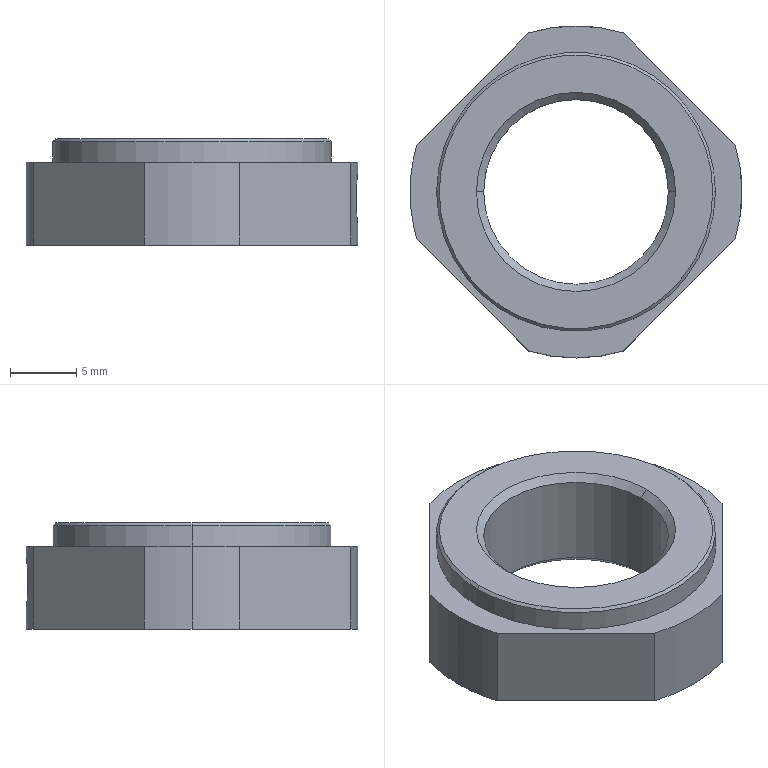Part | NX | features BREP 1 | 1 solid | 34 faces | box 25 x 25 x 8 mm | volume 2054 mm3 | cylinder 13 | cone 12 | plane 9 | commonest cylinder face diameters 25 x5 3.242 x4 13.917 x2 21 x2
STEP:
#1=CARTESIAN_POINT('',(0.,12.121,1.879));
#2=VERTEX_POINT('',#1);
#3=CARTESIAN_POINT('',(0.,7.228,1.879));
#4=VERTEX_POINT('',#3);
#5=CARTESIAN_POINT('',(0.,12.121,1.879));
#6=DIRECTION('',(0.,-1.,0.));
#7=VECTOR('',#6,1000.);
#8=LINE('',#5,#7);
#9=EDGE_CURVE('',#2,#4,#8,.T.);
#10=ORIENTED_EDGE('',*,*,#9,.F.);
#11=CARTESIAN_POINT('',(0.,12.121,5.121));
#12=VERTEX_POINT('',#11);
#13=CARTESIAN_POINT('',(0.,12.121,3.5));
#14=DIRECTION('',(0.,-1.,0.));
#15=DIRECTION('',(0.,0.,1.));
#16=AXIS2_PLACEMENT_3D('',#13,#14,#15);
#17=CIRCLE('',#16,1.621);
#18=EDGE_CURVE('',#12,#2,#17,.T.);
#19=ORIENTED_EDGE('',*,*,#18,.F.);
#20=CARTESIAN_POINT('',(0.,7.228,5.121));
#21=VERTEX_POINT('',#20);
#22=CARTESIAN_POINT('',(0.,12.121,5.121));
#23=DIRECTION('',(0.,-1.,0.));
#24=VECTOR('',#23,1000.);
#25=LINE('',#22,#24);
#26=EDGE_CURVE('',#12,#21,#25,.T.);
#27=ORIENTED_EDGE('',*,*,#26,.T.);
#28=CARTESIAN_POINT('',(0.,7.228,3.5));
#29=DIRECTION('',(0.,1.,0.));
#30=DIRECTION('',(0.,0.,-1.));
#31=AXIS2_PLACEMENT_3D('',#28,#29,#30);
#32=CIRCLE('',#31,1.621);
#33=EDGE_CURVE('',#4,#21,#32,.T.);
#34=ORIENTED_EDGE('',*,*,#33,.F.);
#35=EDGE_LOOP('',(#10,#19,#27,#34));
#36=FACE_BOUND('',#35,.T.);
#37=CARTESIAN_POINT('',(0.,12.5,3.5));
#38=DIRECTION('',(0.,-1.,0.));
#39=DIRECTION('',(0.,0.,1.));
#40=AXIS2_PLACEMENT_3D('',#37,#38,#39);
#41=CYLINDRICAL_SURFACE('',#40,1.621);
#42=ADVANCED_FACE('',(#36),#41,.F.);
#43=ORIENTED_EDGE('',*,*,#33,.T.);
#44=CARTESIAN_POINT('',(0.,7.228,3.5));
#45=DIRECTION('',(0.,1.,0.));
#46=DIRECTION('',(0.,0.,1.));
#47=AXIS2_PLACEMENT_3D('',#44,#45,#46);
#48=CIRCLE('',#47,1.621);
#49=EDGE_CURVE('',#21,#4,#48,.T.);
#50=ORIENTED_EDGE('',*,*,#49,.T.);
#51=EDGE_LOOP('',(#43,#50));
#52=FACE_BOUND('',#51,.T.);
#53=CARTESIAN_POINT('',(0.,7.228,3.5));
#54=DIRECTION('',(0.,1.,0.));
#55=DIRECTION('',(1.,0.,0.));
#56=AXIS2_PLACEMENT_3D('',#53,#54,#55);
#57=PLANE('',#56);
#58=ADVANCED_FACE('',(#52),#57,.T.);
#59=ORIENTED_EDGE('',*,*,#26,.F.);
#60=CARTESIAN_POINT('',(0.,12.121,3.5));
#61=DIRECTION('',(0.,-1.,0.));
#62=DIRECTION('',(0.,0.,-1.));
#63=AXIS2_PLACEMENT_3D('',#60,#61,#62);
#64=CIRCLE('',#63,1.621);
#65=EDGE_CURVE('',#2,#12,#64,.T.);
#66=ORIENTED_EDGE('',*,*,#65,.F.);
#67=ORIENTED_EDGE('',*,*,#9,.T.);
#68=ORIENTED_EDGE('',*,*,#49,.F.);
#69=EDGE_LOOP('',(#59,#66,#67,#68));
#70=FACE_BOUND('',#69,.T.);
#71=CARTESIAN_POINT('',(0.,12.5,3.5));
#72=DIRECTION('',(0.,-1.,0.));
#73=DIRECTION('',(0.,0.,1.));
#74=AXIS2_PLACEMENT_3D('',#71,#72,#73);
#75=CYLINDRICAL_SURFACE('',#74,1.621);
#76=ADVANCED_FACE('',(#70),#75,.F.);
#77=CARTESIAN_POINT('',(-0.0004841,12.5,1.5));
#78=VERTEX_POINT('',#77);
#79=CARTESIAN_POINT('',(0.,12.121,1.879));
#80=CARTESIAN_POINT('',(-0.000003277,12.247,1.753));
#81=CARTESIAN_POINT('',(-0.000007319,12.374,1.626));
#82=CARTESIAN_POINT('',(-0.00001213,12.5,1.5));
#83=B_SPLINE_CURVE_WITH_KNOTS('',3,(#79,#80,#81,#82),.UNSPECIFIED.,.F.,.F.,(4,4),(0.,1.),.UNSPECIFIED.);
#84=EDGE_CURVE('',#78,#2,#83,.F.);
#85=ORIENTED_EDGE('',*,*,#84,.T.);
#86=ORIENTED_EDGE('',*,*,#65,.T.);
#87=CARTESIAN_POINT('',(-0.000000003,12.5,5.5));
#88=VERTEX_POINT('',#87);
#89=CARTESIAN_POINT('',(0.,12.121,5.121));
#90=DIRECTION('',(-0.000000005,0.7071,0.7071));
#91=VECTOR('',#90,1000.);
#92=LINE('',#89,#91);
#93=EDGE_CURVE('',#88,#12,#92,.F.);
#94=ORIENTED_EDGE('',*,*,#93,.F.);
#95=CARTESIAN_POINT('',(1.356,12.426,4.868));
#96=VERTEX_POINT('',#95);
#97=CARTESIAN_POINT('',(1.356,12.426,4.868));
#98=CARTESIAN_POINT('',(0.9975,12.465,5.279));
#99=CARTESIAN_POINT('',(0.5025,12.5,5.5));
#100=CARTESIAN_POINT('',(-0.000000003,12.5,5.5));
#101=B_SPLINE_CURVE_WITH_KNOTS('',3,(#97,#98,#99,#100),.UNSPECIFIED.,.F.,.F.,(4,4),(0.,1.),.UNSPECIFIED.);
#102=EDGE_CURVE('',#96,#88,#101,.T.);
#103=ORIENTED_EDGE('',*,*,#102,.F.);
#104=CARTESIAN_POINT('',(-0.00001213,12.5,1.5));
#105=CARTESIAN_POINT('',(0.6876,12.5,1.5));
#106=CARTESIAN_POINT('',(2.094,12.337,2.407));
#107=CARTESIAN_POINT('',(1.861,12.371,4.289));
#108=CARTESIAN_POINT('',(1.356,12.426,4.868));
#109=B_SPLINE_CURVE_WITH_KNOTS('',3,(#104,#105,#106,#107,#108),.UNSPECIFIED.,.F.,.F.,(4,1,4),(0.,0.5,1.),.UNSPECIFIED.);
#110=EDGE_CURVE('',#78,#96,#109,.T.);
#111=ORIENTED_EDGE('',*,*,#110,.F.);
#112=EDGE_LOOP('',(#85,#86,#94,#103,#111));
#113=FACE_BOUND('',#112,.T.);
#114=CARTESIAN_POINT('',(0.,12.311,3.5));
#115=DIRECTION('',(0.,1.,0.));
#116=DIRECTION('',(0.,0.,1.));
#117=AXIS2_PLACEMENT_3D('',#114,#115,#116);
#118=CONICAL_SURFACE('',#117,1.811,0.7854);
#119=ADVANCED_FACE('',(#113),#118,.F.);
#120=CARTESIAN_POINT('',(-3.58,11.976,0.));
#121=VERTEX_POINT('',#120);
#122=CARTESIAN_POINT('',(-3.58,11.976,6.25));
#123=VERTEX_POINT('',#122);
#124=CARTESIAN_POINT('',(-3.58,11.976,0.));
#125=DIRECTION('',(0.,0.,1.));
#126=VECTOR('',#125,1000.);
#127=LINE('',#124,#126);
#128=EDGE_CURVE('',#121,#123,#127,.T.);
#129=ORIENTED_EDGE('',*,*,#128,.T.);
#130=CARTESIAN_POINT('',(3.58,11.976,6.25));
#131=VERTEX_POINT('',#130);
#132=CARTESIAN_POINT('',(0.,0.,6.25));
#133=DIRECTION('',(0.,0.,1.));
#134=DIRECTION('',(0.2864,0.9581,0.));
#135=AXIS2_PLACEMENT_3D('',#132,#133,#134);
#136=CIRCLE('',#135,12.5);
#137=EDGE_CURVE('',#131,#123,#136,.T.);
#138=ORIENTED_EDGE('',*,*,#137,.F.);
#139=CARTESIAN_POINT('',(3.58,11.976,0.));
#140=VERTEX_POINT('',#139);
#141=CARTESIAN_POINT('',(3.58,11.976,6.25));
#142=DIRECTION('',(0.,0.,-1.));
#143=VECTOR('',#142,1000.);
#144=LINE('',#141,#143);
#145=EDGE_CURVE('',#131,#140,#144,.T.);
#146=ORIENTED_EDGE('',*,*,#145,.T.);
#147=CARTESIAN_POINT('',(0.,0.,0.));
#148=DIRECTION('',(0.,0.,-1.));
#149=DIRECTION('',(-0.2864,0.9581,0.));
#150=AXIS2_PLACEMENT_3D('',#147,#148,#149);
#151=CIRCLE('',#150,12.5);
#152=EDGE_CURVE('',#121,#140,#151,.T.);
#153=ORIENTED_EDGE('',*,*,#152,.F.);
#154=EDGE_LOOP('',(#129,#138,#146,#153));
#155=FACE_BOUND('',#154,.T.);
#156=ORIENTED_EDGE('',*,*,#102,.T.);
#157=CARTESIAN_POINT('',(-1.357,12.426,2.134));
#158=VERTEX_POINT('',#157);
#159=CARTESIAN_POINT('',(-0.000000003,12.5,5.5));
#160=CARTESIAN_POINT('',(-0.6839,12.5,5.5));
#161=CARTESIAN_POINT('',(-2.094,12.337,4.589));
#162=CARTESIAN_POINT('',(-1.865,12.371,2.716));
#163=CARTESIAN_POINT('',(-1.357,12.426,2.134));
#164=B_SPLINE_CURVE_WITH_KNOTS('',3,(#159,#160,#161,#162,#163),.UNSPECIFIED.,.F.,.F.,(4,1,4),(0.,0.5,1.),.UNSPECIFIED.);
#165=EDGE_CURVE('',#88,#158,#164,.T.);
#166=ORIENTED_EDGE('',*,*,#165,.T.);
#167=CARTESIAN_POINT('',(-1.357,12.426,2.134));
#168=CARTESIAN_POINT('',(-1.003,12.465,1.727));
#169=CARTESIAN_POINT('',(-0.5062,12.5,1.5));
#170=CARTESIAN_POINT('',(-0.0004841,12.5,1.5));
#171=B_SPLINE_CURVE_WITH_KNOTS('',3,(#167,#168,#169,#170),.UNSPECIFIED.,.F.,.F.,(4,4),(0.,0.9997),.UNSPECIFIED.);
#172=EDGE_CURVE('',#158,#78,#171,.T.);
#173=ORIENTED_EDGE('',*,*,#172,.T.);
#174=ORIENTED_EDGE('',*,*,#110,.T.);
#175=EDGE_LOOP('',(#156,#166,#173,#174));
#176=FACE_BOUND('',#175,.T.);
#177=CARTESIAN_POINT('',(0.,0.,6.25));
#178=DIRECTION('',(0.,0.,1.));
#179=DIRECTION('',(-1.,0.,0.));
#180=AXIS2_PLACEMENT_3D('',#177,#178,#179);
#181=CYLINDRICAL_SURFACE('',#180,12.5);
#182=ADVANCED_FACE('',(#155,#176),#181,.T.);
#183=ORIENTED_EDGE('',*,*,#152,.T.);
#184=CARTESIAN_POINT('',(11.976,3.58,0.));
#185=VERTEX_POINT('',#184);
#186=CARTESIAN_POINT('',(3.58,11.976,0.));
#187=DIRECTION('',(0.7071,-0.7071,0.));
#188=VECTOR('',#187,1000.);
#189=LINE('',#186,#188);
#190=EDGE_CURVE('',#140,#185,#189,.T.);
#191=ORIENTED_EDGE('',*,*,#190,.T.);
#192=CARTESIAN_POINT('',(11.976,-3.58,0.));
#193=VERTEX_POINT('',#192);
#194=CARTESIAN_POINT('',(0.,0.,0.));
#195=DIRECTION('',(0.,0.,-1.));
#196=DIRECTION('',(0.9581,0.2864,0.));
#197=AXIS2_PLACEMENT_3D('',#194,#195,#196);
#198=CIRCLE('',#197,12.5);
#199=EDGE_CURVE('',#185,#193,#198,.T.);
#200=ORIENTED_EDGE('',*,*,#199,.T.);
#201=CARTESIAN_POINT('',(3.58,-11.976,0.));
#202=VERTEX_POINT('',#201);
#203=CARTESIAN_POINT('',(11.976,-3.58,0.));
#204=DIRECTION('',(-0.7071,-0.7071,0.));
#205=VECTOR('',#204,1000.);
#206=LINE('',#203,#205);
#207=EDGE_CURVE('',#193,#202,#206,.T.);
#208=ORIENTED_EDGE('',*,*,#207,.T.);
#209=CARTESIAN_POINT('',(-3.58,-11.976,0.));
#210=VERTEX_POINT('',#209);
#211=CARTESIAN_POINT('',(0.,0.,0.));
#212=DIRECTION('',(0.,0.,-1.));
#213=DIRECTION('',(0.2864,-0.9581,0.));
#214=AXIS2_PLACEMENT_3D('',#211,#212,#213);
#215=CIRCLE('',#214,12.5);
#216=EDGE_CURVE('',#202,#210,#215,.T.);
#217=ORIENTED_EDGE('',*,*,#216,.T.);
#218=CARTESIAN_POINT('',(-11.976,-3.58,0.));
#219=VERTEX_POINT('',#218);
#220=CARTESIAN_POINT('',(-3.58,-11.976,0.));
#221=DIRECTION('',(-0.7071,0.7071,0.));
#222=VECTOR('',#221,1000.);
#223=LINE('',#220,#222);
#224=EDGE_CURVE('',#210,#219,#223,.T.);
#225=ORIENTED_EDGE('',*,*,#224,.T.);
#226=CARTESIAN_POINT('',(-12.5,0.,0.));
#227=VERTEX_POINT('',#226);
#228=CARTESIAN_POINT('',(0.,0.,0.));
#229=DIRECTION('',(0.,0.,-1.));
#230=DIRECTION('',(-0.9581,-0.2864,0.));
#231=AXIS2_PLACEMENT_3D('',#228,#229,#230);
#232=CIRCLE('',#231,12.5);
#233=EDGE_CURVE('',#219,#227,#232,.T.);
#234=ORIENTED_EDGE('',*,*,#233,.T.);
#235=CARTESIAN_POINT('',(-11.976,3.58,0.));
#236=VERTEX_POINT('',#235);
#237=CARTESIAN_POINT('',(0.,0.,0.));
#238=DIRECTION('',(0.,0.,-1.));
#239=DIRECTION('',(-0.9581,-0.2864,0.));
#240=AXIS2_PLACEMENT_3D('',#237,#238,#239);
#241=CIRCLE('',#240,12.5);
#242=EDGE_CURVE('',#227,#236,#241,.T.);
#243=ORIENTED_EDGE('',*,*,#242,.T.);
#244=CARTESIAN_POINT('',(-11.976,3.58,0.));
#245=DIRECTION('',(0.7071,0.7071,0.));
#246=VECTOR('',#245,1000.);
#247=LINE('',#244,#246);
#248=EDGE_CURVE('',#236,#121,#247,.T.);
#249=ORIENTED_EDGE('',*,*,#248,.T.);
#250=EDGE_LOOP('',(#183,#191,#200,#208,#217,#225,#234,#243,#249));
#251=FACE_BOUND('',#250,.T.);
#252=CARTESIAN_POINT('',(7.5,0.,0.));
#253=VERTEX_POINT('',#252);
#254=CARTESIAN_POINT('',(-7.5,0.,0.));
#255=VERTEX_POINT('',#254);
#256=CARTESIAN_POINT('',(0.,0.,0.));
#257=DIRECTION('',(0.,0.,1.));
#258=DIRECTION('',(1.,0.,0.));
#259=AXIS2_PLACEMENT_3D('',#256,#257,#258);
#260=CIRCLE('',#259,7.5);
#261=EDGE_CURVE('',#253,#255,#260,.T.);
#262=ORIENTED_EDGE('',*,*,#261,.T.);
#263=CARTESIAN_POINT('',(0.,0.,0.));
#264=DIRECTION('',(0.,0.,1.));
#265=DIRECTION('',(-1.,0.,0.));
#266=AXIS2_PLACEMENT_3D('',#263,#264,#265);
#267=CIRCLE('',#266,7.5);
#268=EDGE_CURVE('',#255,#253,#267,.T.);
#269=ORIENTED_EDGE('',*,*,#268,.T.);
#270=EDGE_LOOP('',(#262,#269));
#271=FACE_BOUND('',#270,.T.);
#272=CARTESIAN_POINT('',(0.,0.,0.));
#273=DIRECTION('',(0.,0.,1.));
#274=DIRECTION('',(1.,0.,0.));
#275=AXIS2_PLACEMENT_3D('',#272,#273,#274);
#276=PLANE('',#275);
#277=ADVANCED_FACE('',(#251,#271),#276,.F.);
#278=CARTESIAN_POINT('',(-11.976,3.58,6.25));
#279=VERTEX_POINT('',#278);
#280=CARTESIAN_POINT('',(-11.976,3.58,6.25));
#281=DIRECTION('',(0.,0.,-1.));
#282=VECTOR('',#281,1000.);
#283=LINE('',#280,#282);
#284=EDGE_CURVE('',#279,#236,#283,.T.);
#285=ORIENTED_EDGE('',*,*,#284,.F.);
#286=CARTESIAN_POINT('',(-3.58,11.976,6.25));
#287=DIRECTION('',(-0.7071,-0.7071,0.));
#288=VECTOR('',#287,1000.);
#289=LINE('',#286,#288);
#290=EDGE_CURVE('',#123,#279,#289,.T.);
#291=ORIENTED_EDGE('',*,*,#290,.F.);
#292=ORIENTED_EDGE('',*,*,#128,.F.);
#293=ORIENTED_EDGE('',*,*,#248,.F.);
#294=EDGE_LOOP('',(#285,#291,#292,#293));
#295=FACE_BOUND('',#294,.T.);
#296=CARTESIAN_POINT('',(-3.58,11.976,6.25));
#297=DIRECTION('',(0.7071,-0.7071,0.));
#298=DIRECTION('',(0.,0.,-1.));
#299=AXIS2_PLACEMENT_3D('',#296,#297,#298);
#300=PLANE('',#299);
#301=ADVANCED_FACE('',(#295),#300,.F.);
#302=CARTESIAN_POINT('',(-12.5,0.,6.25));
#303=VERTEX_POINT('',#302);
#304=CARTESIAN_POINT('',(0.,0.,6.25));
#305=DIRECTION('',(0.,0.,1.));
#306=DIRECTION('',(-0.9581,0.2864,0.));
#307=AXIS2_PLACEMENT_3D('',#304,#305,#306);
#308=CIRCLE('',#307,12.5);
#309=EDGE_CURVE('',#279,#303,#308,.T.);
#310=ORIENTED_EDGE('',*,*,#309,.T.);
#311=CARTESIAN_POINT('',(-11.976,-3.58,6.25));
#312=VERTEX_POINT('',#311);
#313=CARTESIAN_POINT('',(0.,0.,6.25));
#314=DIRECTION('',(0.,0.,1.));
#315=DIRECTION('',(-0.9581,0.2864,0.));
#316=AXIS2_PLACEMENT_3D('',#313,#314,#315);
#317=CIRCLE('',#316,12.5);
#318=EDGE_CURVE('',#303,#312,#317,.T.);
#319=ORIENTED_EDGE('',*,*,#318,.T.);
#320=CARTESIAN_POINT('',(-3.58,-11.976,6.25));
#321=VERTEX_POINT('',#320);
#322=CARTESIAN_POINT('',(-11.976,-3.58,6.25));
#323=DIRECTION('',(0.7071,-0.7071,0.));
#324=VECTOR('',#323,1000.);
#325=LINE('',#322,#324);
#326=EDGE_CURVE('',#312,#321,#325,.T.);
#327=ORIENTED_EDGE('',*,*,#326,.T.);
#328=CARTESIAN_POINT('',(3.58,-11.976,6.25));
#329=VERTEX_POINT('',#328);
#330=CARTESIAN_POINT('',(0.,0.,6.25));
#331=DIRECTION('',(0.,0.,1.));
#332=DIRECTION('',(-0.2864,-0.9581,0.));
#333=AXIS2_PLACEMENT_3D('',#330,#331,#332);
#334=CIRCLE('',#333,12.5);
#335=EDGE_CURVE('',#321,#329,#334,.T.);
#336=ORIENTED_EDGE('',*,*,#335,.T.);
#337=CARTESIAN_POINT('',(11.976,-3.58,6.25));
#338=VERTEX_POINT('',#337);
#339=CARTESIAN_POINT('',(3.58,-11.976,6.25));
#340=DIRECTION('',(0.7071,0.7071,0.));
#341=VECTOR('',#340,1000.);
#342=LINE('',#339,#341);
#343=EDGE_CURVE('',#329,#338,#342,.T.);
#344=ORIENTED_EDGE('',*,*,#343,.T.);
#345=CARTESIAN_POINT('',(11.976,3.58,6.25));
#346=VERTEX_POINT('',#345);
#347=CARTESIAN_POINT('',(0.,0.,6.25));
#348=DIRECTION('',(0.,0.,1.));
#349=DIRECTION('',(0.9581,-0.2864,0.));
#350=AXIS2_PLACEMENT_3D('',#347,#348,#349);
#351=CIRCLE('',#350,12.5);
#352=EDGE_CURVE('',#338,#346,#351,.T.);
#353=ORIENTED_EDGE('',*,*,#352,.T.);
#354=CARTESIAN_POINT('',(11.976,3.58,6.25));
#355=DIRECTION('',(-0.7071,0.7071,0.));
#356=VECTOR('',#355,1000.);
#357=LINE('',#354,#356);
#358=EDGE_CURVE('',#346,#131,#357,.T.);
#359=ORIENTED_EDGE('',*,*,#358,.T.);
#360=ORIENTED_EDGE('',*,*,#137,.T.);
#361=ORIENTED_EDGE('',*,*,#290,.T.);
#362=EDGE_LOOP('',(#310,#319,#327,#336,#344,#353,#359,#360,#361));
#363=FACE_BOUND('',#362,.T.);
#364=CARTESIAN_POINT('',(-10.5,0.,6.25));
#365=VERTEX_POINT('',#364);
#366=CARTESIAN_POINT('',(10.5,0.,6.25));
#367=VERTEX_POINT('',#366);
#368=CARTESIAN_POINT('',(0.,0.,6.25));
#369=DIRECTION('',(0.,0.,-1.));
#370=DIRECTION('',(-1.,0.,0.));
#371=AXIS2_PLACEMENT_3D('',#368,#369,#370);
#372=CIRCLE('',#371,10.5);
#373=EDGE_CURVE('',#365,#367,#372,.T.);
#374=ORIENTED_EDGE('',*,*,#373,.T.);
#375=CARTESIAN_POINT('',(0.,0.,6.25));
#376=DIRECTION('',(0.,0.,-1.));
#377=DIRECTION('',(1.,0.,0.));
#378=AXIS2_PLACEMENT_3D('',#375,#376,#377);
#379=CIRCLE('',#378,10.5);
#380=EDGE_CURVE('',#367,#365,#379,.T.);
#381=ORIENTED_EDGE('',*,*,#380,.T.);
#382=EDGE_LOOP('',(#374,#381));
#383=FACE_BOUND('',#382,.T.);
#384=CARTESIAN_POINT('',(0.,0.,6.25));
#385=DIRECTION('',(0.,0.,1.));
#386=DIRECTION('',(1.,0.,0.));
#387=AXIS2_PLACEMENT_3D('',#384,#385,#386);
#388=PLANE('',#387);
#389=ADVANCED_FACE('',(#363,#383),#388,.T.);
#390=ORIENTED_EDGE('',*,*,#145,.F.);
#391=ORIENTED_EDGE('',*,*,#358,.F.);
#392=CARTESIAN_POINT('',(11.976,3.58,0.));
#393=DIRECTION('',(0.,0.,1.));
#394=VECTOR('',#393,1000.);
#395=LINE('',#392,#394);
#396=EDGE_CURVE('',#185,#346,#395,.T.);
#397=ORIENTED_EDGE('',*,*,#396,.F.);
#398=ORIENTED_EDGE('',*,*,#190,.F.);
#399=EDGE_LOOP('',(#390,#391,#397,#398));
#400=FACE_BOUND('',#399,.T.);
#401=CARTESIAN_POINT('',(11.976,3.58,6.25));
#402=DIRECTION('',(-0.7071,-0.7071,0.));
#403=DIRECTION('',(-0.7071,0.7071,0.));
#404=AXIS2_PLACEMENT_3D('',#401,#402,#403);
#405=PLANE('',#404);
#406=ADVANCED_FACE('',(#400),#405,.F.);
#407=ORIENTED_EDGE('',*,*,#396,.T.);
#408=ORIENTED_EDGE('',*,*,#352,.F.);
#409=CARTESIAN_POINT('',(11.976,-3.58,6.25));
#410=DIRECTION('',(0.,0.,-1.));
#411=VECTOR('',#410,1000.);
#412=LINE('',#409,#411);
#413=EDGE_CURVE('',#338,#193,#412,.T.);
#414=ORIENTED_EDGE('',*,*,#413,.T.);
#415=ORIENTED_EDGE('',*,*,#199,.F.);
#416=EDGE_LOOP('',(#407,#408,#414,#415));
#417=FACE_BOUND('',#416,.T.);
#418=CARTESIAN_POINT('',(12.5,0.,5.5));
#419=VERTEX_POINT('',#418);
#420=CARTESIAN_POINT('',(12.426,1.358,4.865));
#421=VERTEX_POINT('',#420);
#422=CARTESIAN_POINT('',(12.5,0.,5.5));
#423=CARTESIAN_POINT('',(12.5,0.51,5.5));
#424=CARTESIAN_POINT('',(12.464,1.008,5.267));
#425=CARTESIAN_POINT('',(12.426,1.358,4.865));
#426=B_SPLINE_CURVE_WITH_KNOTS('',3,(#422,#423,#424,#425),.UNSPECIFIED.,.F.,.F.,(4,4),(0.,1.),.UNSPECIFIED.);
#427=EDGE_CURVE('',#419,#421,#426,.T.);
#428=ORIENTED_EDGE('',*,*,#427,.T.);
#429=CARTESIAN_POINT('',(12.5,0.,1.5));
#430=VERTEX_POINT('',#429);
#431=CARTESIAN_POINT('',(12.426,1.358,4.865));
#432=CARTESIAN_POINT('',(12.371,1.861,4.288));
#433=CARTESIAN_POINT('',(12.333,2.115,2.461));
#434=CARTESIAN_POINT('',(12.5,0.6906,1.5));
#435=CARTESIAN_POINT('',(12.5,0.,1.5));
#436=B_SPLINE_CURVE_WITH_KNOTS('',3,(#431,#432,#433,#434,#435),.UNSPECIFIED.,.F.,.F.,(4,1,4),(0.,0.5,1.),.UNSPECIFIED.);
#437=EDGE_CURVE('',#421,#430,#436,.T.);
#438=ORIENTED_EDGE('',*,*,#437,.T.);
#439=CARTESIAN_POINT('',(12.426,-1.357,2.134));
#440=VERTEX_POINT('',#439);
#441=CARTESIAN_POINT('',(12.5,0.,1.5));
#442=CARTESIAN_POINT('',(12.5,-0.4987,1.5));
#443=CARTESIAN_POINT('',(12.465,-1.003,1.727));
#444=CARTESIAN_POINT('',(12.426,-1.357,2.134));
#445=B_SPLINE_CURVE_WITH_KNOTS('',3,(#441,#442,#443,#444),.UNSPECIFIED.,.F.,.F.,(4,4),(0.,1.),.UNSPECIFIED.);
#446=EDGE_CURVE('',#430,#440,#445,.T.);
#447=ORIENTED_EDGE('',*,*,#446,.T.);
#448=CARTESIAN_POINT('',(12.426,-1.357,2.134));
#449=CARTESIAN_POINT('',(12.371,-1.865,2.716));
#450=CARTESIAN_POINT('',(12.334,-2.114,4.546));
#451=CARTESIAN_POINT('',(12.5,-0.6815,5.5));
#452=CARTESIAN_POINT('',(12.5,0.,5.5));
#453=B_SPLINE_CURVE_WITH_KNOTS('',3,(#448,#449,#450,#451,#452),.UNSPECIFIED.,.F.,.F.,(4,1,4),(0.,0.5,1.),.UNSPECIFIED.);
#454=EDGE_CURVE('',#440,#419,#453,.T.);
#455=ORIENTED_EDGE('',*,*,#454,.T.);
#456=EDGE_LOOP('',(#428,#438,#447,#455));
#457=FACE_BOUND('',#456,.T.);
#458=CARTESIAN_POINT('',(0.,0.,6.25));
#459=DIRECTION('',(0.,0.,1.));
#460=DIRECTION('',(-1.,0.,0.));
#461=AXIS2_PLACEMENT_3D('',#458,#459,#460);
#462=CYLINDRICAL_SURFACE('',#461,12.5);
#463=ADVANCED_FACE('',(#417,#457),#462,.T.);
#464=ORIENTED_EDGE('',*,*,#413,.F.);
#465=ORIENTED_EDGE('',*,*,#343,.F.);
#466=CARTESIAN_POINT('',(3.58,-11.976,0.));
#467=DIRECTION('',(0.,0.,1.));
#468=VECTOR('',#467,1000.);
#469=LINE('',#466,#468);
#470=EDGE_CURVE('',#202,#329,#469,.T.);
#471=ORIENTED_EDGE('',*,*,#470,.F.);
#472=ORIENTED_EDGE('',*,*,#207,.F.);
#473=EDGE_LOOP('',(#464,#465,#471,#472));
#474=FACE_BOUND('',#473,.T.);
#475=CARTESIAN_POINT('',(3.58,-11.976,6.25));
#476=DIRECTION('',(-0.7071,0.7071,0.));
#477=DIRECTION('',(0.,0.,1.));
#478=AXIS2_PLACEMENT_3D('',#475,#476,#477);
#479=PLANE('',#478);
#480=ADVANCED_FACE('',(#474),#479,.F.);
#481=ORIENTED_EDGE('',*,*,#470,.T.);
#482=ORIENTED_EDGE('',*,*,#335,.F.);
#483=CARTESIAN_POINT('',(-3.58,-11.976,6.25));
#484=DIRECTION('',(0.,0.,-1.));
#485=VECTOR('',#484,1000.);
#486=LINE('',#483,#485);
#487=EDGE_CURVE('',#321,#210,#486,.T.);
#488=ORIENTED_EDGE('',*,*,#487,.T.);
#489=ORIENTED_EDGE('',*,*,#216,.F.);
#490=EDGE_LOOP('',(#481,#482,#488,#489));
#491=FACE_BOUND('',#490,.T.);
#492=CARTESIAN_POINT('',(0.,0.,6.25));
#493=DIRECTION('',(0.,0.,1.));
#494=DIRECTION('',(-1.,0.,0.));
#495=AXIS2_PLACEMENT_3D('',#492,#493,#494);
#496=CYLINDRICAL_SURFACE('',#495,12.5);
#497=ADVANCED_FACE('',(#491),#496,.T.);
#498=ORIENTED_EDGE('',*,*,#487,.F.);
#499=ORIENTED_EDGE('',*,*,#326,.F.);
#500=CARTESIAN_POINT('',(-11.976,-3.58,0.));
#501=DIRECTION('',(0.,0.,1.));
#502=VECTOR('',#501,1000.);
#503=LINE('',#500,#502);
#504=EDGE_CURVE('',#219,#312,#503,.T.);
#505=ORIENTED_EDGE('',*,*,#504,.F.);
#506=ORIENTED_EDGE('',*,*,#224,.F.);
#507=EDGE_LOOP('',(#498,#499,#505,#506));
#508=FACE_BOUND('',#507,.T.);
#509=CARTESIAN_POINT('',(-11.976,-3.58,6.25));
#510=DIRECTION('',(0.7071,0.7071,0.));
#511=DIRECTION('',(0.,0.,-1.));
#512=AXIS2_PLACEMENT_3D('',#509,#510,#511);
#513=PLANE('',#512);
#514=ADVANCED_FACE('',(#508),#513,.F.);
#515=CARTESIAN_POINT('',(-12.5,0.,6.25));
#516=DIRECTION('',(0.,0.,1.));
#517=VECTOR('',#516,1000.);
#518=LINE('',#515,#517);
#519=EDGE_CURVE('',#227,#303,#518,.T.);
#520=ORIENTED_EDGE('',*,*,#519,.F.);
#521=ORIENTED_EDGE('',*,*,#233,.F.);
#522=ORIENTED_EDGE('',*,*,#504,.T.);
#523=ORIENTED_EDGE('',*,*,#318,.F.);
#524=EDGE_LOOP('',(#520,#521,#522,#523));
#525=FACE_BOUND('',#524,.T.);
#526=CARTESIAN_POINT('',(0.,0.,6.25));
#527=DIRECTION('',(0.,0.,1.));
#528=DIRECTION('',(-1.,0.,0.));
#529=AXIS2_PLACEMENT_3D('',#526,#527,#528);
#530=CYLINDRICAL_SURFACE('',#529,12.5);
#531=ADVANCED_FACE('',(#525),#530,.T.);
#532=CARTESIAN_POINT('',(12.121,0.,1.879));
#533=VERTEX_POINT('',#532);
#534=CARTESIAN_POINT('',(12.121,0.,1.879));
#535=DIRECTION('',(0.7071,0.,-0.7071));
#536=VECTOR('',#535,1000.);
#537=LINE('',#534,#536);
#538=EDGE_CURVE('',#533,#430,#537,.T.);
#539=ORIENTED_EDGE('',*,*,#538,.F.);
#540=CARTESIAN_POINT('',(12.121,0.,5.121));
#541=VERTEX_POINT('',#540);
#542=CARTESIAN_POINT('',(12.121,0.,3.5));
#543=DIRECTION('',(-1.,0.,0.));
#544=DIRECTION('',(0.,0.,-1.));
#545=AXIS2_PLACEMENT_3D('',#542,#543,#544);
#546=CIRCLE('',#545,1.621);
#547=EDGE_CURVE('',#533,#541,#546,.T.);
#548=ORIENTED_EDGE('',*,*,#547,.T.);
#549=CARTESIAN_POINT('',(12.121,0.,5.121));
#550=DIRECTION('',(0.7071,0.,0.7071));
#551=VECTOR('',#550,1000.);
#552=LINE('',#549,#551);
#553=EDGE_CURVE('',#541,#419,#552,.T.);
#554=ORIENTED_EDGE('',*,*,#553,.T.);
#555=ORIENTED_EDGE('',*,*,#454,.F.);
#556=ORIENTED_EDGE('',*,*,#446,.F.);
#557=EDGE_LOOP('',(#539,#548,#554,#555,#556));
#558=FACE_BOUND('',#557,.T.);
#559=CARTESIAN_POINT('',(12.31,0.,3.5));
#560=DIRECTION('',(1.,0.,0.));
#561=DIRECTION('',(0.,0.,-1.));
#562=AXIS2_PLACEMENT_3D('',#559,#560,#561);
#563=CONICAL_SURFACE('',#562,1.81,0.7854);
#564=ADVANCED_FACE('',(#558),#563,.F.);
#565=ORIENTED_EDGE('',*,*,#427,.F.);
#566=ORIENTED_EDGE('',*,*,#553,.F.);
#567=CARTESIAN_POINT('',(12.121,0.,3.5));
#568=DIRECTION('',(-1.,0.,0.));
#569=DIRECTION('',(0.,0.,1.));
#570=AXIS2_PLACEMENT_3D('',#567,#568,#569);
#571=CIRCLE('',#570,1.621);
#572=EDGE_CURVE('',#541,#533,#571,.T.);
#573=ORIENTED_EDGE('',*,*,#572,.T.);
#574=ORIENTED_EDGE('',*,*,#538,.T.);
#575=ORIENTED_EDGE('',*,*,#437,.F.);
#576=EDGE_LOOP('',(#565,#566,#573,#574,#575));
#577=FACE_BOUND('',#576,.T.);
#578=CARTESIAN_POINT('',(12.31,0.,3.5));
#579=DIRECTION('',(1.,0.,0.));
#580=DIRECTION('',(0.,0.,-1.));
#581=AXIS2_PLACEMENT_3D('',#578,#579,#580);
#582=CONICAL_SURFACE('',#581,1.81,0.7854);
#583=ADVANCED_FACE('',(#577),#582,.F.);
#584=CARTESIAN_POINT('',(7.607,0.,5.121));
#585=VERTEX_POINT('',#584);
#586=CARTESIAN_POINT('',(7.607,0.,5.121));
#587=DIRECTION('',(1.,0.,0.));
#588=VECTOR('',#587,1000.);
#589=LINE('',#586,#588);
#590=EDGE_CURVE('',#541,#585,#589,.F.);
#591=ORIENTED_EDGE('',*,*,#590,.T.);
#592=CARTESIAN_POINT('',(7.607,0.,1.879));
#593=VERTEX_POINT('',#592);
#594=CARTESIAN_POINT('',(7.607,0.,3.5));
#595=DIRECTION('',(1.,0.,0.));
#596=DIRECTION('',(0.,0.,-1.));
#597=AXIS2_PLACEMENT_3D('',#594,#595,#596);
#598=CIRCLE('',#597,1.621);
#599=EDGE_CURVE('',#593,#585,#598,.T.);
#600=ORIENTED_EDGE('',*,*,#599,.F.);
#601=CARTESIAN_POINT('',(7.607,0.,1.879));
#602=DIRECTION('',(1.,0.,0.));
#603=VECTOR('',#602,1000.);
#604=LINE('',#601,#603);
#605=EDGE_CURVE('',#533,#593,#604,.F.);
#606=ORIENTED_EDGE('',*,*,#605,.F.);
#607=ORIENTED_EDGE('',*,*,#572,.F.);
#608=EDGE_LOOP('',(#591,#600,#606,#607));
#609=FACE_BOUND('',#608,.T.);
#610=CARTESIAN_POINT('',(7.228,0.,3.5));
#611=DIRECTION('',(1.,0.,0.));
#612=DIRECTION('',(0.,0.,1.));
#613=AXIS2_PLACEMENT_3D('',#610,#611,#612);
#614=CYLINDRICAL_SURFACE('',#613,1.621);
#615=ADVANCED_FACE('',(#609),#614,.F.);
#616=ORIENTED_EDGE('',*,*,#605,.T.);
#617=CARTESIAN_POINT('',(7.607,0.,3.5));
#618=DIRECTION('',(1.,0.,0.));
#619=DIRECTION('',(0.,0.,1.));
#620=AXIS2_PLACEMENT_3D('',#617,#618,#619);
#621=CIRCLE('',#620,1.621);
#622=EDGE_CURVE('',#585,#593,#621,.T.);
#623=ORIENTED_EDGE('',*,*,#622,.F.);
#624=ORIENTED_EDGE('',*,*,#590,.F.);
#625=ORIENTED_EDGE('',*,*,#547,.F.);
#626=EDGE_LOOP('',(#616,#623,#624,#625));
#627=FACE_BOUND('',#626,.T.);
#628=CARTESIAN_POINT('',(7.228,0.,3.5));
#629=DIRECTION('',(1.,0.,0.));
#630=DIRECTION('',(0.,0.,1.));
#631=AXIS2_PLACEMENT_3D('',#628,#629,#630);
#632=CYLINDRICAL_SURFACE('',#631,1.621);
#633=ADVANCED_FACE('',(#627),#632,.F.);
#634=CARTESIAN_POINT('',(7.228,0.,5.5));
#635=VERTEX_POINT('',#634);
#636=CARTESIAN_POINT('',(7.607,0.,5.121));
#637=DIRECTION('',(-0.7071,0.,0.7071));
#638=VECTOR('',#637,1000.);
#639=LINE('',#636,#638);
#640=EDGE_CURVE('',#635,#585,#639,.F.);
#641=ORIENTED_EDGE('',*,*,#640,.T.);
#642=ORIENTED_EDGE('',*,*,#622,.T.);
#643=CARTESIAN_POINT('',(7.228,0.,1.5));
#644=VERTEX_POINT('',#643);
#645=CARTESIAN_POINT('',(7.607,0.,1.879));
#646=DIRECTION('',(-0.7071,0.,-0.7071));
#647=VECTOR('',#646,1000.);
#648=LINE('',#645,#647);
#649=EDGE_CURVE('',#644,#593,#648,.F.);
#650=ORIENTED_EDGE('',*,*,#649,.F.);
#651=CARTESIAN_POINT('',(7.228,0.,3.5));
#652=DIRECTION('',(1.,0.,0.));
#653=DIRECTION('',(0.,0.,1.));
#654=AXIS2_PLACEMENT_3D('',#651,#652,#653);
#655=CIRCLE('',#654,2.);
#656=EDGE_CURVE('',#635,#644,#655,.T.);
#657=ORIENTED_EDGE('',*,*,#656,.F.);
#658=EDGE_LOOP('',(#641,#642,#650,#657));
#659=FACE_BOUND('',#658,.T.);
#660=CARTESIAN_POINT('',(7.418,0.,3.5));
#661=DIRECTION('',(-1.,0.,0.));
#662=DIRECTION('',(0.,0.,1.));
#663=AXIS2_PLACEMENT_3D('',#660,#661,#662);
#664=CONICAL_SURFACE('',#663,1.811,0.7854);
#665=ADVANCED_FACE('',(#659),#664,.F.);
#666=CARTESIAN_POINT('',(7.228,0.,3.5));
#667=DIRECTION('',(1.,0.,0.));
#668=DIRECTION('',(0.,0.,-1.));
#669=AXIS2_PLACEMENT_3D('',#666,#667,#668);
#670=CIRCLE('',#669,2.);
#671=EDGE_CURVE('',#644,#635,#670,.T.);
#672=ORIENTED_EDGE('',*,*,#671,.T.);
#673=ORIENTED_EDGE('',*,*,#656,.T.);
#674=EDGE_LOOP('',(#672,#673));
#675=FACE_BOUND('',#674,.T.);
#676=CARTESIAN_POINT('',(7.228,0.,5.5));
#677=DIRECTION('',(1.,0.,0.));
#678=DIRECTION('',(0.,1.,0.));
#679=AXIS2_PLACEMENT_3D('',#676,#677,#678);
#680=PLANE('',#679);
#681=ADVANCED_FACE('',(#675),#680,.T.);
#682=ORIENTED_EDGE('',*,*,#649,.T.);
#683=ORIENTED_EDGE('',*,*,#599,.T.);
#684=ORIENTED_EDGE('',*,*,#640,.F.);
#685=ORIENTED_EDGE('',*,*,#671,.F.);
#686=EDGE_LOOP('',(#682,#683,#684,#685));
#687=FACE_BOUND('',#686,.T.);
#688=CARTESIAN_POINT('',(7.418,0.,3.5));
#689=DIRECTION('',(-1.,0.,0.));
#690=DIRECTION('',(0.,0.,1.));
#691=AXIS2_PLACEMENT_3D('',#688,#689,#690);
#692=CONICAL_SURFACE('',#691,1.811,0.7854);
#693=ADVANCED_FACE('',(#687),#692,.F.);
#694=CARTESIAN_POINT('',(-10.5,0.,7.8));
#695=VERTEX_POINT('',#694);
#696=CARTESIAN_POINT('',(-10.5,0.,6.25));
#697=DIRECTION('',(0.,0.,1.));
#698=VECTOR('',#697,1000.);
#699=LINE('',#696,#698);
#700=EDGE_CURVE('',#365,#695,#699,.T.);
#701=ORIENTED_EDGE('',*,*,#700,.F.);
#702=ORIENTED_EDGE('',*,*,#380,.F.);
#703=CARTESIAN_POINT('',(10.5,0.,7.8));
#704=VERTEX_POINT('',#703);
#705=CARTESIAN_POINT('',(10.5,0.,6.25));
#706=DIRECTION('',(0.,0.,1.));
#707=VECTOR('',#706,1000.);
#708=LINE('',#705,#707);
#709=EDGE_CURVE('',#367,#704,#708,.T.);
#710=ORIENTED_EDGE('',*,*,#709,.T.);
#711=CARTESIAN_POINT('',(0.,0.,7.8));
#712=DIRECTION('',(0.,0.,1.));
#713=DIRECTION('',(-1.,0.,0.));
#714=AXIS2_PLACEMENT_3D('',#711,#712,#713);
#715=CIRCLE('',#714,10.5);
#716=EDGE_CURVE('',#695,#704,#715,.T.);
#717=ORIENTED_EDGE('',*,*,#716,.F.);
#718=EDGE_LOOP('',(#701,#702,#710,#717));
#719=FACE_BOUND('',#718,.T.);
#720=CARTESIAN_POINT('',(0.,0.,0.));
#721=DIRECTION('',(0.,0.,1.));
#722=DIRECTION('',(-1.,0.,0.));
#723=AXIS2_PLACEMENT_3D('',#720,#721,#722);
#724=CYLINDRICAL_SURFACE('',#723,10.5);
#725=ADVANCED_FACE('',(#719),#724,.T.);
#726=CARTESIAN_POINT('',(10.3,0.,8.));
#727=VERTEX_POINT('',#726);
#728=CARTESIAN_POINT('',(10.3,0.,8.));
#729=DIRECTION('',(0.7071,0.,-0.7071));
#730=VECTOR('',#729,1000.);
#731=LINE('',#728,#730);
#732=EDGE_CURVE('',#704,#727,#731,.F.);
#733=ORIENTED_EDGE('',*,*,#732,.T.);
#734=CARTESIAN_POINT('',(-10.3,0.,8.));
#735=VERTEX_POINT('',#734);
#736=CARTESIAN_POINT('',(0.,0.,8.));
#737=DIRECTION('',(0.,0.,1.));
#738=DIRECTION('',(-1.,0.,0.));
#739=AXIS2_PLACEMENT_3D('',#736,#737,#738);
#740=CIRCLE('',#739,10.3);
#741=EDGE_CURVE('',#735,#727,#740,.T.);
#742=ORIENTED_EDGE('',*,*,#741,.F.);
#743=CARTESIAN_POINT('',(-10.3,0.,8.));
#744=DIRECTION('',(-0.7071,0.,-0.7071));
#745=VECTOR('',#744,1000.);
#746=LINE('',#743,#745);
#747=EDGE_CURVE('',#695,#735,#746,.F.);
#748=ORIENTED_EDGE('',*,*,#747,.F.);
#749=ORIENTED_EDGE('',*,*,#716,.T.);
#750=EDGE_LOOP('',(#733,#742,#748,#749));
#751=FACE_BOUND('',#750,.T.);
#752=CARTESIAN_POINT('',(0.,0.,7.9));
#753=DIRECTION('',(0.,0.,-1.));
#754=DIRECTION('',(-1.,0.,0.));
#755=AXIS2_PLACEMENT_3D('',#752,#753,#754);
#756=CONICAL_SURFACE('',#755,10.4,0.7854);
#757=ADVANCED_FACE('',(#751),#756,.T.);
#758=ORIENTED_EDGE('',*,*,#747,.T.);
#759=CARTESIAN_POINT('',(0.,0.,8.));
#760=DIRECTION('',(0.,0.,1.));
#761=DIRECTION('',(1.,0.,0.));
#762=AXIS2_PLACEMENT_3D('',#759,#760,#761);
#763=CIRCLE('',#762,10.3);
#764=EDGE_CURVE('',#727,#735,#763,.T.);
#765=ORIENTED_EDGE('',*,*,#764,.F.);
#766=ORIENTED_EDGE('',*,*,#732,.F.);
#767=CARTESIAN_POINT('',(0.,0.,7.8));
#768=DIRECTION('',(0.,0.,1.));
#769=DIRECTION('',(1.,0.,0.));
#770=AXIS2_PLACEMENT_3D('',#767,#768,#769);
#771=CIRCLE('',#770,10.5);
#772=EDGE_CURVE('',#704,#695,#771,.T.);
#773=ORIENTED_EDGE('',*,*,#772,.T.);
#774=EDGE_LOOP('',(#758,#765,#766,#773));
#775=FACE_BOUND('',#774,.T.);
#776=CARTESIAN_POINT('',(0.,0.,7.9));
#777=DIRECTION('',(0.,0.,-1.));
#778=DIRECTION('',(-1.,0.,0.));
#779=AXIS2_PLACEMENT_3D('',#776,#777,#778);
#780=CONICAL_SURFACE('',#779,10.4,0.7854);
#781=ADVANCED_FACE('',(#775),#780,.T.);
#782=ORIENTED_EDGE('',*,*,#709,.F.);
#783=ORIENTED_EDGE('',*,*,#373,.F.);
#784=ORIENTED_EDGE('',*,*,#700,.T.);
#785=ORIENTED_EDGE('',*,*,#772,.F.);
#786=EDGE_LOOP('',(#782,#783,#784,#785));
#787=FACE_BOUND('',#786,.T.);
#788=CARTESIAN_POINT('',(0.,0.,0.));
#789=DIRECTION('',(0.,0.,1.));
#790=DIRECTION('',(-1.,0.,0.));
#791=AXIS2_PLACEMENT_3D('',#788,#789,#790);
#792=CYLINDRICAL_SURFACE('',#791,10.5);
#793=ADVANCED_FACE('',(#787),#792,.T.);
#794=ORIENTED_EDGE('',*,*,#764,.T.);
#795=ORIENTED_EDGE('',*,*,#741,.T.);
#796=EDGE_LOOP('',(#794,#795));
#797=FACE_BOUND('',#796,.T.);
#798=CARTESIAN_POINT('',(7.5,0.,8.));
#799=VERTEX_POINT('',#798);
#800=CARTESIAN_POINT('',(-7.5,0.,8.));
#801=VERTEX_POINT('',#800);
#802=CARTESIAN_POINT('',(0.,0.,8.));
#803=DIRECTION('',(0.,0.,-1.));
#804=DIRECTION('',(1.,0.,0.));
#805=AXIS2_PLACEMENT_3D('',#802,#803,#804);
#806=CIRCLE('',#805,7.5);
#807=EDGE_CURVE('',#799,#801,#806,.T.);
#808=ORIENTED_EDGE('',*,*,#807,.T.);
#809=CARTESIAN_POINT('',(0.,0.,8.));
#810=DIRECTION('',(0.,0.,-1.));
#811=DIRECTION('',(-1.,0.,0.));
#812=AXIS2_PLACEMENT_3D('',#809,#810,#811);
#813=CIRCLE('',#812,7.5);
#814=EDGE_CURVE('',#801,#799,#813,.T.);
#815=ORIENTED_EDGE('',*,*,#814,.T.);
#816=EDGE_LOOP('',(#808,#815));
#817=FACE_BOUND('',#816,.T.);
#818=CARTESIAN_POINT('',(0.,0.,8.));
#819=DIRECTION('',(0.,0.,-1.));
#820=DIRECTION('',(0.,-1.,0.));
#821=AXIS2_PLACEMENT_3D('',#818,#819,#820);
#822=PLANE('',#821);
#823=ADVANCED_FACE('',(#797,#817),#822,.F.);
#824=CARTESIAN_POINT('',(-6.958,0.,7.459));
#825=VERTEX_POINT('',#824);
#826=CARTESIAN_POINT('',(-6.958,0.,7.459));
#827=DIRECTION('',(-0.7071,0.,0.7071));
#828=VECTOR('',#827,1000.);
#829=LINE('',#826,#828);
#830=EDGE_CURVE('',#825,#801,#829,.T.);
#831=ORIENTED_EDGE('',*,*,#830,.F.);
#832=CARTESIAN_POINT('',(6.958,0.,7.459));
#833=VERTEX_POINT('',#832);
#834=CARTESIAN_POINT('',(0.,0.,7.459));
#835=DIRECTION('',(0.,0.,-1.));
#836=DIRECTION('',(-1.,0.,0.));
#837=AXIS2_PLACEMENT_3D('',#834,#835,#836);
#838=CIRCLE('',#837,6.958);
#839=EDGE_CURVE('',#825,#833,#838,.T.);
#840=ORIENTED_EDGE('',*,*,#839,.T.);
#841=CARTESIAN_POINT('',(6.958,0.,7.459));
#842=DIRECTION('',(0.7071,0.,0.7071));
#843=VECTOR('',#842,1000.);
#844=LINE('',#841,#843);
#845=EDGE_CURVE('',#833,#799,#844,.T.);
#846=ORIENTED_EDGE('',*,*,#845,.T.);
#847=ORIENTED_EDGE('',*,*,#814,.F.);
#848=EDGE_LOOP('',(#831,#840,#846,#847));
#849=FACE_BOUND('',#848,.T.);
#850=CARTESIAN_POINT('',(0.,0.,7.729));
#851=DIRECTION('',(0.,0.,1.));
#852=DIRECTION('',(1.,0.,0.));
#853=AXIS2_PLACEMENT_3D('',#850,#851,#852);
#854=CONICAL_SURFACE('',#853,7.229,0.7854);
#855=ADVANCED_FACE('',(#849),#854,.F.);
#856=ORIENTED_EDGE('',*,*,#845,.F.);
#857=CARTESIAN_POINT('',(0.,0.,7.459));
#858=DIRECTION('',(0.,0.,-1.));
#859=DIRECTION('',(1.,0.,0.));
#860=AXIS2_PLACEMENT_3D('',#857,#858,#859);
#861=CIRCLE('',#860,6.958);
#862=EDGE_CURVE('',#833,#825,#861,.T.);
#863=ORIENTED_EDGE('',*,*,#862,.T.);
#864=ORIENTED_EDGE('',*,*,#830,.T.);
#865=ORIENTED_EDGE('',*,*,#807,.F.);
#866=EDGE_LOOP('',(#856,#863,#864,#865));
#867=FACE_BOUND('',#866,.T.);
#868=CARTESIAN_POINT('',(0.,0.,7.729));
#869=DIRECTION('',(0.,0.,1.));
#870=DIRECTION('',(1.,0.,0.));
#871=AXIS2_PLACEMENT_3D('',#868,#869,#870);
#872=CONICAL_SURFACE('',#871,7.229,0.7854);
#873=ADVANCED_FACE('',(#867),#872,.F.);
#874=CARTESIAN_POINT('',(6.958,0.,0.5415));
#875=VERTEX_POINT('',#874);
#876=CARTESIAN_POINT('',(6.958,0.,0.5415));
#877=DIRECTION('',(0.,0.,1.));
#878=VECTOR('',#877,1000.);
#879=LINE('',#876,#878);
#880=EDGE_CURVE('',#833,#875,#879,.F.);
#881=ORIENTED_EDGE('',*,*,#880,.T.);
#882=CARTESIAN_POINT('',(-6.958,0.,0.5415));
#883=VERTEX_POINT('',#882);
#884=CARTESIAN_POINT('',(0.,0.,0.5415));
#885=DIRECTION('',(0.,0.,1.));
#886=DIRECTION('',(-1.,0.,0.));
#887=AXIS2_PLACEMENT_3D('',#884,#885,#886);
#888=CIRCLE('',#887,6.958);
#889=EDGE_CURVE('',#883,#875,#888,.T.);
#890=ORIENTED_EDGE('',*,*,#889,.F.);
#891=CARTESIAN_POINT('',(-6.958,0.,0.5415));
#892=DIRECTION('',(0.,0.,1.));
#893=VECTOR('',#892,1000.);
#894=LINE('',#891,#893);
#895=EDGE_CURVE('',#825,#883,#894,.F.);
#896=ORIENTED_EDGE('',*,*,#895,.F.);
#897=ORIENTED_EDGE('',*,*,#862,.F.);
#898=EDGE_LOOP('',(#881,#890,#896,#897));
#899=FACE_BOUND('',#898,.T.);
#900=CARTESIAN_POINT('',(0.,0.,0.));
#901=DIRECTION('',(0.,0.,1.));
#902=DIRECTION('',(-1.,0.,0.));
#903=AXIS2_PLACEMENT_3D('',#900,#901,#902);
#904=CYLINDRICAL_SURFACE('',#903,6.958);
#905=ADVANCED_FACE('',(#899),#904,.F.);
#906=ORIENTED_EDGE('',*,*,#895,.T.);
#907=CARTESIAN_POINT('',(0.,0.,0.5415));
#908=DIRECTION('',(0.,0.,1.));
#909=DIRECTION('',(1.,0.,0.));
#910=AXIS2_PLACEMENT_3D('',#907,#908,#909);
#911=CIRCLE('',#910,6.958);
#912=EDGE_CURVE('',#875,#883,#911,.T.);
#913=ORIENTED_EDGE('',*,*,#912,.F.);
#914=ORIENTED_EDGE('',*,*,#880,.F.);
#915=ORIENTED_EDGE('',*,*,#839,.F.);
#916=EDGE_LOOP('',(#906,#913,#914,#915));
#917=FACE_BOUND('',#916,.T.);
#918=CARTESIAN_POINT('',(0.,0.,0.));
#919=DIRECTION('',(0.,0.,1.));
#920=DIRECTION('',(-1.,0.,0.));
#921=AXIS2_PLACEMENT_3D('',#918,#919,#920);
#922=CYLINDRICAL_SURFACE('',#921,6.958);
#923=ADVANCED_FACE('',(#917),#922,.F.);
#924=CARTESIAN_POINT('',(6.958,0.,0.5415));
#925=DIRECTION('',(0.7071,0.,-0.7071));
#926=VECTOR('',#925,1000.);
#927=LINE('',#924,#926);
#928=EDGE_CURVE('',#253,#875,#927,.F.);
#929=ORIENTED_EDGE('',*,*,#928,.T.);
#930=ORIENTED_EDGE('',*,*,#912,.T.);
#931=CARTESIAN_POINT('',(-6.958,0.,0.5415));
#932=DIRECTION('',(-0.7071,0.,-0.7071));
#933=VECTOR('',#932,1000.);
#934=LINE('',#931,#933);
#935=EDGE_CURVE('',#255,#883,#934,.F.);
#936=ORIENTED_EDGE('',*,*,#935,.F.);
#937=ORIENTED_EDGE('',*,*,#261,.F.);
#938=EDGE_LOOP('',(#929,#930,#936,#937));
#939=FACE_BOUND('',#938,.T.);
#940=CARTESIAN_POINT('',(0.,0.,0.2707));
#941=DIRECTION('',(0.,0.,-1.));
#942=DIRECTION('',(-1.,0.,0.));
#943=AXIS2_PLACEMENT_3D('',#940,#941,#942);
#944=CONICAL_SURFACE('',#943,7.229,0.7854);
#945=ADVANCED_FACE('',(#939),#944,.F.);
#946=ORIENTED_EDGE('',*,*,#935,.T.);
#947=ORIENTED_EDGE('',*,*,#889,.T.);
#948=ORIENTED_EDGE('',*,*,#928,.F.);
#949=ORIENTED_EDGE('',*,*,#268,.F.);
#950=EDGE_LOOP('',(#946,#947,#948,#949));
#951=FACE_BOUND('',#950,.T.);
#952=CARTESIAN_POINT('',(0.,0.,0.2707));
#953=DIRECTION('',(0.,0.,-1.));
#954=DIRECTION('',(-1.,0.,0.));
#955=AXIS2_PLACEMENT_3D('',#952,#953,#954);
#956=CONICAL_SURFACE('',#955,7.229,0.7854);
#957=ADVANCED_FACE('',(#951),#956,.F.);
#958=ORIENTED_EDGE('',*,*,#93,.T.);
#959=ORIENTED_EDGE('',*,*,#18,.T.);
#960=ORIENTED_EDGE('',*,*,#84,.F.);
#961=ORIENTED_EDGE('',*,*,#172,.F.);
#962=ORIENTED_EDGE('',*,*,#165,.F.);
#963=EDGE_LOOP('',(#958,#959,#960,#961,#962));
#964=FACE_BOUND('',#963,.T.);
#965=CARTESIAN_POINT('',(0.,12.311,3.5));
#966=DIRECTION('',(0.,1.,0.));
#967=DIRECTION('',(0.,0.,1.));
#968=AXIS2_PLACEMENT_3D('',#965,#966,#967);
#969=CONICAL_SURFACE('',#968,1.811,0.7854);
#970=ADVANCED_FACE('',(#964),#969,.F.);
#971=ORIENTED_EDGE('',*,*,#242,.F.);
#972=ORIENTED_EDGE('',*,*,#519,.T.);
#973=ORIENTED_EDGE('',*,*,#309,.F.);
#974=ORIENTED_EDGE('',*,*,#284,.T.);
#975=EDGE_LOOP('',(#971,#972,#973,#974));
#976=FACE_BOUND('',#975,.T.);
#977=CARTESIAN_POINT('',(0.,0.,6.25));
#978=DIRECTION('',(0.,0.,1.));
#979=DIRECTION('',(-1.,0.,0.));
#980=AXIS2_PLACEMENT_3D('',#977,#978,#979);
#981=CYLINDRICAL_SURFACE('',#980,12.5);
#982=ADVANCED_FACE('',(#976),#981,.T.);
#983=CLOSED_SHELL('',(#42,#58,#76,#119,#182,#277,#301,#389,#406,#463,#480,#497,#514,#531,#564,#583,#615,#633,#665,#681,#693,#725,#757,#781,#793,#823,#855,#873,#905,#923,#945,#957,#970,#982));
#984=MANIFOLD_SOLID_BREP('',#983);
#985=(LENGTH_UNIT()NAMED_UNIT(*)SI_UNIT(.MILLI.,.METRE.));
#986=UNCERTAINTY_MEASURE_WITH_UNIT(LENGTH_MEASURE(0.0508),#985,'','');
#987=(NAMED_UNIT(*)PLANE_ANGLE_UNIT()SI_UNIT($,.RADIAN.));
#988=(NAMED_UNIT(*)SI_UNIT($,.STERADIAN.)SOLID_ANGLE_UNIT());
#989=(GEOMETRIC_REPRESENTATION_CONTEXT(3)GLOBAL_UNCERTAINTY_ASSIGNED_CONTEXT((#986))GLOBAL_UNIT_ASSIGNED_CONTEXT((#985,#987,#988))REPRESENTATION_CONTEXT('',''));
#990=ADVANCED_BREP_SHAPE_REPRESENTATION('',(#984),#989);